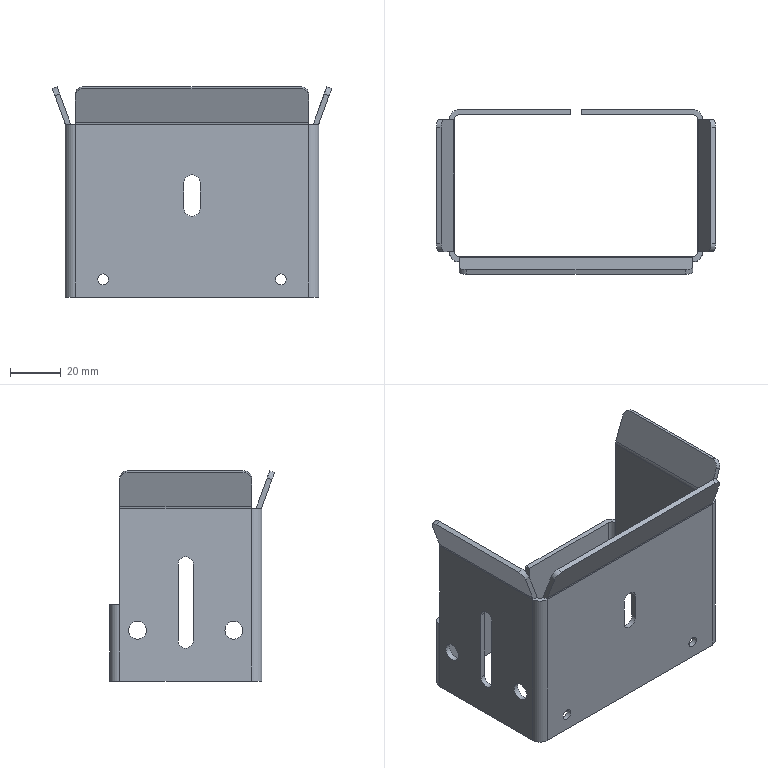Part | NX | features M5 螺纹孔1 2 | 1 solid | 72 faces | box 110.019 x 65.01 x 82.801 mm | volume 38324 mm3 | plane 38 | cylinder 34 | commonest cylinder face diameters 6 x10 4 x7 8 x7 4.2 x4 7 x4 6.4 x2